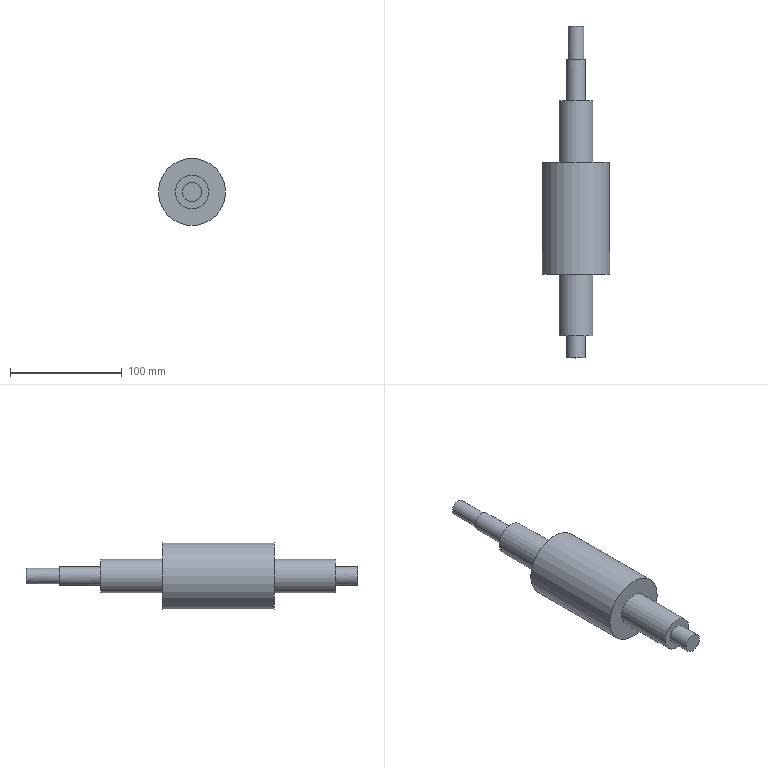Part | STEP file | 冲床-300配套压波_id310_x_t | 1 solid | 13 faces | box 60 x 297 x 60 mm | volume 378054 mm3 | plane 7 | cylinder 6 | commonest cylinder face diameters 17 x2 30 x2 14 x1 60 x1
STEP:
#1=CARTESIAN_POINT('',(1130.,-50.,125.));
#2=VERTEX_POINT('',#1);
#3=CARTESIAN_POINT('',(1130.,-50.,110.));
#4=DIRECTION('',(0.,-1.,0.));
#5=DIRECTION('',(0.,0.,1.));
#6=AXIS2_PLACEMENT_3D('',#3,#4,#5);
#7=CIRCLE('',#6,15.);
#8=EDGE_CURVE('',#2,#2,#7,.T.);
#9=ORIENTED_EDGE('',*,*,#8,.F.);
#10=EDGE_LOOP('',(#9));
#11=FACE_BOUND('',#10,.T.);
#12=CARTESIAN_POINT('',(1160.,-50.,110.));
#13=VERTEX_POINT('',#12);
#14=CARTESIAN_POINT('',(1130.,-50.,110.));
#15=DIRECTION('',(0.,1.,0.));
#16=DIRECTION('',(1.,0.,0.));
#17=AXIS2_PLACEMENT_3D('',#14,#15,#16);
#18=CIRCLE('',#17,30.);
#19=EDGE_CURVE('',#13,#13,#18,.T.);
#20=ORIENTED_EDGE('',*,*,#19,.F.);
#21=EDGE_LOOP('',(#20));
#22=FACE_BOUND('',#21,.T.);
#23=CARTESIAN_POINT('',(1300.,-50.,24.7));
#24=DIRECTION('',(0.,-1.,0.));
#25=DIRECTION('',(-1.,0.,0.));
#26=AXIS2_PLACEMENT_3D('',#23,#24,#25);
#27=PLANE('',#26);
#28=ADVANCED_FACE('',(#11,#22),#27,.T.);
#29=CARTESIAN_POINT('',(1130.,50.,125.));
#30=VERTEX_POINT('',#29);
#31=CARTESIAN_POINT('',(1130.,50.,110.));
#32=DIRECTION('',(0.,1.,0.));
#33=DIRECTION('',(0.,0.,1.));
#34=AXIS2_PLACEMENT_3D('',#31,#32,#33);
#35=CIRCLE('',#34,15.);
#36=EDGE_CURVE('',#30,#30,#35,.T.);
#37=ORIENTED_EDGE('',*,*,#36,.F.);
#38=EDGE_LOOP('',(#37));
#39=FACE_BOUND('',#38,.T.);
#40=CARTESIAN_POINT('',(1100.,50.,110.));
#41=VERTEX_POINT('',#40);
#42=CARTESIAN_POINT('',(1130.,50.,110.));
#43=DIRECTION('',(0.,-1.,0.));
#44=DIRECTION('',(-1.,0.,0.));
#45=AXIS2_PLACEMENT_3D('',#42,#43,#44);
#46=CIRCLE('',#45,30.);
#47=EDGE_CURVE('',#41,#41,#46,.T.);
#48=ORIENTED_EDGE('',*,*,#47,.F.);
#49=EDGE_LOOP('',(#48));
#50=FACE_BOUND('',#49,.T.);
#51=CARTESIAN_POINT('',(1300.,50.,24.7));
#52=DIRECTION('',(0.,1.,0.));
#53=DIRECTION('',(-1.,0.,0.));
#54=AXIS2_PLACEMENT_3D('',#51,#52,#53);
#55=PLANE('',#54);
#56=ADVANCED_FACE('',(#39,#50),#55,.T.);
#57=ORIENTED_EDGE('',*,*,#47,.T.);
#58=EDGE_LOOP('',(#57));
#59=FACE_BOUND('',#58,.T.);
#60=ORIENTED_EDGE('',*,*,#19,.T.);
#61=EDGE_LOOP('',(#60));
#62=FACE_BOUND('',#61,.T.);
#63=CARTESIAN_POINT('',(1130.,-3333.3,110.));
#64=DIRECTION('',(0.,1.,0.));
#65=DIRECTION('',(0.,0.,1.));
#66=AXIS2_PLACEMENT_3D('',#63,#64,#65);
#67=CYLINDRICAL_SURFACE('',#66,30.);
#68=ADVANCED_FACE('',(#59,#62),#67,.T.);
#69=ORIENTED_EDGE('',*,*,#36,.T.);
#70=EDGE_LOOP('',(#69));
#71=FACE_BOUND('',#70,.T.);
#72=CARTESIAN_POINT('',(1130.,105.,125.));
#73=VERTEX_POINT('',#72);
#74=CARTESIAN_POINT('',(1130.,105.,110.));
#75=DIRECTION('',(0.,1.,0.));
#76=DIRECTION('',(0.,0.,1.));
#77=AXIS2_PLACEMENT_3D('',#74,#75,#76);
#78=CIRCLE('',#77,15.);
#79=EDGE_CURVE('',#73,#73,#78,.T.);
#80=ORIENTED_EDGE('',*,*,#79,.F.);
#81=EDGE_LOOP('',(#80));
#82=FACE_BOUND('',#81,.T.);
#83=CARTESIAN_POINT('',(1130.,50.,110.));
#84=DIRECTION('',(0.,1.,0.));
#85=DIRECTION('',(-1.,0.,0.));
#86=AXIS2_PLACEMENT_3D('',#83,#84,#85);
#87=CYLINDRICAL_SURFACE('',#86,15.);
#88=ADVANCED_FACE('',(#71,#82),#87,.T.);
#89=CARTESIAN_POINT('',(1130.,105.,118.5));
#90=VERTEX_POINT('',#89);
#91=CARTESIAN_POINT('',(1130.,105.,110.));
#92=DIRECTION('',(0.,-1.,0.));
#93=DIRECTION('',(0.,0.,1.));
#94=AXIS2_PLACEMENT_3D('',#91,#92,#93);
#95=CIRCLE('',#94,8.5);
#96=EDGE_CURVE('',#90,#90,#95,.T.);
#97=ORIENTED_EDGE('',*,*,#96,.T.);
#98=EDGE_LOOP('',(#97));
#99=FACE_BOUND('',#98,.T.);
#100=ORIENTED_EDGE('',*,*,#79,.T.);
#101=EDGE_LOOP('',(#100));
#102=FACE_BOUND('',#101,.T.);
#103=CARTESIAN_POINT('',(1130.,105.,110.));
#104=DIRECTION('',(0.,1.,0.));
#105=DIRECTION('',(0.,0.,1.));
#106=AXIS2_PLACEMENT_3D('',#103,#104,#105);
#107=PLANE('',#106);
#108=ADVANCED_FACE('',(#99,#102),#107,.T.);
#109=CARTESIAN_POINT('',(1138.5,142.,110.));
#110=VERTEX_POINT('',#109);
#111=CARTESIAN_POINT('',(1130.,142.,110.));
#112=DIRECTION('',(0.,-1.,0.));
#113=DIRECTION('',(1.,0.,0.));
#114=AXIS2_PLACEMENT_3D('',#111,#112,#113);
#115=CIRCLE('',#114,8.5);
#116=EDGE_CURVE('',#110,#110,#115,.T.);
#117=ORIENTED_EDGE('',*,*,#116,.T.);
#118=EDGE_LOOP('',(#117));
#119=FACE_BOUND('',#118,.T.);
#120=ORIENTED_EDGE('',*,*,#96,.F.);
#121=EDGE_LOOP('',(#120));
#122=FACE_BOUND('',#121,.T.);
#123=CARTESIAN_POINT('',(1130.,80.,110.));
#124=DIRECTION('',(0.,1.,0.));
#125=DIRECTION('',(0.,0.,1.));
#126=AXIS2_PLACEMENT_3D('',#123,#124,#125);
#127=CYLINDRICAL_SURFACE('',#126,8.5);
#128=ADVANCED_FACE('',(#119,#122),#127,.T.);
#129=ORIENTED_EDGE('',*,*,#8,.T.);
#130=EDGE_LOOP('',(#129));
#131=FACE_BOUND('',#130,.T.);
#132=CARTESIAN_POINT('',(1130.,-105.,125.));
#133=VERTEX_POINT('',#132);
#134=CARTESIAN_POINT('',(1130.,-105.,110.));
#135=DIRECTION('',(0.,-1.,0.));
#136=DIRECTION('',(0.,0.,1.));
#137=AXIS2_PLACEMENT_3D('',#134,#135,#136);
#138=CIRCLE('',#137,15.);
#139=EDGE_CURVE('',#133,#133,#138,.T.);
#140=ORIENTED_EDGE('',*,*,#139,.F.);
#141=EDGE_LOOP('',(#140));
#142=FACE_BOUND('',#141,.T.);
#143=CARTESIAN_POINT('',(1130.,-50.,110.));
#144=DIRECTION('',(0.,-1.,0.));
#145=DIRECTION('',(-1.,0.,0.));
#146=AXIS2_PLACEMENT_3D('',#143,#144,#145);
#147=CYLINDRICAL_SURFACE('',#146,15.);
#148=ADVANCED_FACE('',(#131,#142),#147,.T.);
#149=CARTESIAN_POINT('',(1130.,-105.,118.5));
#150=VERTEX_POINT('',#149);
#151=CARTESIAN_POINT('',(1130.,-105.,110.));
#152=DIRECTION('',(0.,1.,0.));
#153=DIRECTION('',(0.,0.,1.));
#154=AXIS2_PLACEMENT_3D('',#151,#152,#153);
#155=CIRCLE('',#154,8.5);
#156=EDGE_CURVE('',#150,#150,#155,.T.);
#157=ORIENTED_EDGE('',*,*,#156,.T.);
#158=EDGE_LOOP('',(#157));
#159=FACE_BOUND('',#158,.T.);
#160=ORIENTED_EDGE('',*,*,#139,.T.);
#161=EDGE_LOOP('',(#160));
#162=FACE_BOUND('',#161,.T.);
#163=CARTESIAN_POINT('',(1130.,-105.,110.));
#164=DIRECTION('',(0.,-1.,0.));
#165=DIRECTION('',(0.,0.,1.));
#166=AXIS2_PLACEMENT_3D('',#163,#164,#165);
#167=PLANE('',#166);
#168=ADVANCED_FACE('',(#159,#162),#167,.T.);
#169=ORIENTED_EDGE('',*,*,#156,.F.);
#170=EDGE_LOOP('',(#169));
#171=FACE_BOUND('',#170,.T.);
#172=CARTESIAN_POINT('',(1121.5,-125.,110.));
#173=VERTEX_POINT('',#172);
#174=CARTESIAN_POINT('',(1130.,-125.,110.));
#175=DIRECTION('',(0.,1.,0.));
#176=DIRECTION('',(-1.,0.,0.));
#177=AXIS2_PLACEMENT_3D('',#174,#175,#176);
#178=CIRCLE('',#177,8.5);
#179=EDGE_CURVE('',#173,#173,#178,.T.);
#180=ORIENTED_EDGE('',*,*,#179,.T.);
#181=EDGE_LOOP('',(#180));
#182=FACE_BOUND('',#181,.T.);
#183=CARTESIAN_POINT('',(1130.,-80.,110.));
#184=DIRECTION('',(0.,-1.,0.));
#185=DIRECTION('',(0.,0.,1.));
#186=AXIS2_PLACEMENT_3D('',#183,#184,#185);
#187=CYLINDRICAL_SURFACE('',#186,8.5);
#188=ADVANCED_FACE('',(#171,#182),#187,.T.);
#189=ORIENTED_EDGE('',*,*,#179,.F.);
#190=EDGE_LOOP('',(#189));
#191=FACE_OUTER_BOUND('',#190,.T.);
#192=CARTESIAN_POINT('',(1155.,-125.,150.));
#193=DIRECTION('',(0.,1.,0.));
#194=DIRECTION('',(0.,0.,-1.));
#195=AXIS2_PLACEMENT_3D('',#192,#193,#194);
#196=PLANE('',#195);
#197=ADVANCED_FACE('',(#191),#196,.F.);
#198=CARTESIAN_POINT('',(1137.,142.,110.));
#199=VERTEX_POINT('',#198);
#200=CARTESIAN_POINT('',(1130.,142.,110.));
#201=DIRECTION('',(0.,1.,0.));
#202=DIRECTION('',(1.,0.,0.));
#203=AXIS2_PLACEMENT_3D('',#200,#201,#202);
#204=CIRCLE('',#203,7.);
#205=EDGE_CURVE('',#199,#199,#204,.T.);
#206=ORIENTED_EDGE('',*,*,#205,.F.);
#207=EDGE_LOOP('',(#206));
#208=FACE_BOUND('',#207,.T.);
#209=ORIENTED_EDGE('',*,*,#116,.F.);
#210=EDGE_LOOP('',(#209));
#211=FACE_BOUND('',#210,.T.);
#212=CARTESIAN_POINT('',(1130.,142.,110.));
#213=DIRECTION('',(0.,-1.,0.));
#214=DIRECTION('',(1.,0.,0.));
#215=AXIS2_PLACEMENT_3D('',#212,#213,#214);
#216=PLANE('',#215);
#217=ADVANCED_FACE('',(#208,#211),#216,.F.);
#218=CARTESIAN_POINT('',(1130.,172.,103.));
#219=VERTEX_POINT('',#218);
#220=CARTESIAN_POINT('',(1130.,172.,110.));
#221=DIRECTION('',(0.,-1.,0.));
#222=DIRECTION('',(0.,0.,-1.));
#223=AXIS2_PLACEMENT_3D('',#220,#221,#222);
#224=CIRCLE('',#223,7.);
#225=EDGE_CURVE('',#219,#219,#224,.T.);
#226=ORIENTED_EDGE('',*,*,#225,.F.);
#227=EDGE_LOOP('',(#226));
#228=FACE_OUTER_BOUND('',#227,.T.);
#229=CARTESIAN_POINT('',(1130.,172.,110.));
#230=DIRECTION('',(0.,-1.,0.));
#231=DIRECTION('',(0.,0.,-1.));
#232=AXIS2_PLACEMENT_3D('',#229,#230,#231);
#233=PLANE('',#232);
#234=ADVANCED_FACE('',(#228),#233,.F.);
#235=ORIENTED_EDGE('',*,*,#225,.T.);
#236=EDGE_LOOP('',(#235));
#237=FACE_BOUND('',#236,.T.);
#238=ORIENTED_EDGE('',*,*,#205,.T.);
#239=EDGE_LOOP('',(#238));
#240=FACE_BOUND('',#239,.T.);
#241=CARTESIAN_POINT('',(1130.,80.,110.));
#242=DIRECTION('',(0.,1.,0.));
#243=DIRECTION('',(0.,0.,1.));
#244=AXIS2_PLACEMENT_3D('',#241,#242,#243);
#245=CYLINDRICAL_SURFACE('',#244,7.);
#246=ADVANCED_FACE('',(#237,#240),#245,.T.);
#247=CLOSED_SHELL('',(#28,#56,#68,#88,#108,#128,#148,#168,#188,#197,#217,#234,#246));
#248=MANIFOLD_SOLID_BREP('',#247);
#249=(LENGTH_UNIT()NAMED_UNIT(*)SI_UNIT(.MILLI.,.METRE.));
#250=UNCERTAINTY_MEASURE_WITH_UNIT(LENGTH_MEASURE(0.00002),#249,'','');
#251=(NAMED_UNIT(*)PLANE_ANGLE_UNIT()SI_UNIT($,.RADIAN.));
#252=PLANE_ANGLE_MEASURE_WITH_UNIT(PLANE_ANGLE_MEASURE(0.01745),#251);
#253=DIMENSIONAL_EXPONENTS(0.,0.,0.,0.,0.,0.,0.);
#254=(CONVERSION_BASED_UNIT('DEGREE',#252)NAMED_UNIT(#253)PLANE_ANGLE_UNIT());
#255=(NAMED_UNIT(*)SI_UNIT($,.STERADIAN.)SOLID_ANGLE_UNIT());
#256=(GEOMETRIC_REPRESENTATION_CONTEXT(3)GLOBAL_UNCERTAINTY_ASSIGNED_CONTEXT((#250))GLOBAL_UNIT_ASSIGNED_CONTEXT((#249,#254,#255))REPRESENTATION_CONTEXT('',''));
#257=ADVANCED_BREP_SHAPE_REPRESENTATION('',(#248),#256);